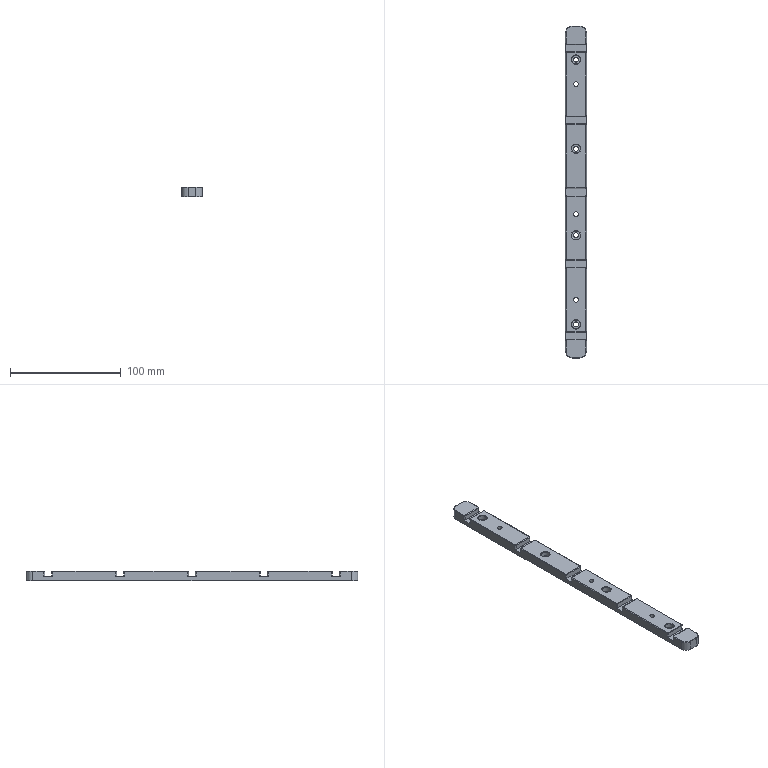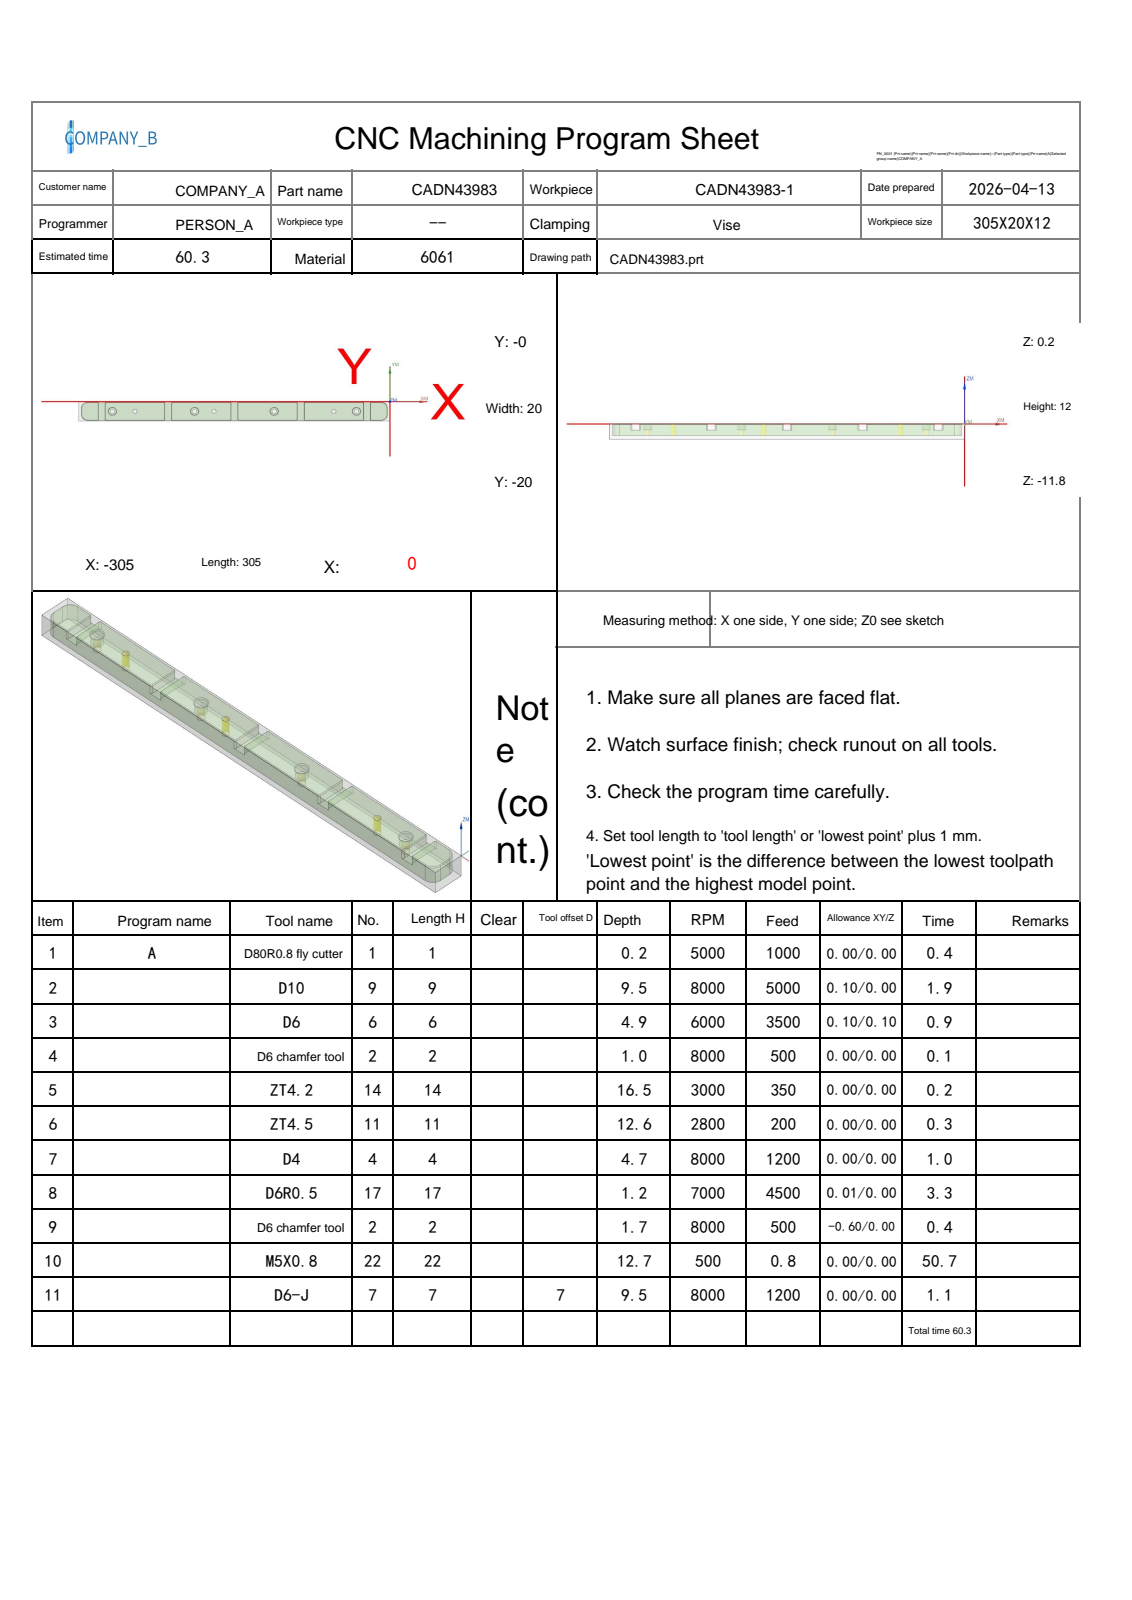NC program | NX | posted by the shop | part box 19 x 300 x 9 mm
Lines 1454 to 2850 of 20188:
N8 T17 M06
(D6R0.5  D=6. R=0.5 H=17 ce=0.01 di=0.00)
G00 G90 G54 X-.332 Y-12.302 M03 S7000
G43 H17 Z20.
M08
Z1.5
G01 Y-13.5 Z1.437 F4500.
Y-13.786 Z1.422
X-.395 Y-14.549 Z1.382
X-.529 Y-15.304 Z1.342
X-.733 Y-16.043 Z1.302
X-1.005 Y-16.759 Z1.262
X-1.344 Y-17.447 Z1.221
X-1.745 Y-18.1 Z1.181
X-2.205 Y-18.712 Z1.141
X-2.721 Y-19.279 Z1.101
X-3.288 Y-19.795 Z1.061
X-3.9 Y-20.255 Z1.021
X-4.553 Y-20.656 Z.98
X-5.241 Y-20.995 Z.94
X-5.957 Y-21.267 Z.9
X-6.696 Y-21.471 Z.86
X-7.45 Y-21.605 Z.82
X-8.214 Y-21.668 Z.78
X-18.528 Z.239
X-18.986 Y-21.608 Z.215
X-19.431 Y-21.482 Z.191
X-19.853 Y-21.294 Z.166
X-20.243 Y-21.046 Z.142
X-20.593 Y-20.743 Z.118
X-20.896 Y-20.393 Z.094
X-21.144 Y-20.003 Z.07
X-21.332 Y-19.581 Z.045
X-21.458 Y-19.136 Z.021
X-21.518 Y-18.678 Z-.003
Y-18.5 Z-.012
Y-1.5
G02 X-18.35 Y1.668 I3.168 J0.0
G01 X-8.5
G02 X-.332 Y-6.5 I0.0 J-8.168
G01 Y-13.5
G02 X-8.5 Y-21.668 I-8.168 J0.0
G01 X-18.35
G02 X-21.518 Y-18.5 I0.0 J3.168
G01 X-21.521 Y-15.667 Z-.013
X-21.527 Y-12.833 Z-.014
X-21.53 Y-10. Z-.015
X-21.536 Y-7.167 Z-.016
X-21.54 Y-4.333
X-21.544 Y-1.5 Z-.017
X-21.543 Y-1.41
X-21.539 Y-1.321
X-21.533 Y-1.231
X-21.524 Y-1.142
X-21.514 Y-1.053
X-21.499 Y-.965
X-21.484 Y-.877
X-21.465 Y-.789
X-21.444 Y-.702
X-21.42 Y-.616
X-21.395 Y-.53
X-21.366 Y-.445
X-21.336 Y-.36 Z-.018
X-21.302 Y-.277
X-21.268 Y-.194
X-21.229 Y-.113
X-21.19 Y-.033
X-21.147 Y.046
X-21.103 Y.124
X-21.056 Y.201
X-21.008 Y.276
X-20.957 Y.35
X-20.905 Y.423
X-20.849 Y.493
X-20.793 Y.563
X-20.734 Y.63
X-20.674 Y.697
X-20.611 Y.761
X-20.547 Y.824
X-20.481 Y.884
X-20.413 Y.944
X-20.344 Y1.
X-20.273 Y1.056
X-20.201 Y1.108
X-20.127 Y1.16
X-20.052 Y1.208
X-19.975 Y1.255
X-19.897 Y1.299
X-19.818 Y1.342
X-19.738 Y1.382
X-19.657 Y1.421
X-19.574 Y1.456
X-19.491 Y1.489
X-19.407 Y1.52
X-19.322 Y1.549
X-19.236 Y1.575
X-19.149 Y1.599
X-19.062 Y1.62
X-18.974 Y1.639
X-18.886 Y1.655
X-18.797 Y1.669
X-18.708 Y1.68
X-18.619 Y1.69
X-18.529 Y1.696 Z-.019
X-18.44 Y1.7
X-18.35 Y1.701
X-15.888 Y1.705
X-13.425 Y1.708 Z-.02
X-10.963 Y1.712 Z-.021
X-8.5 Y1.715
X-8.22 Y1.71
X-7.939 Y1.697
X-7.66 Y1.673 Z-.022
X-7.381 Y1.64
X-7.104 Y1.597
X-6.828 Y1.545
X-6.554 Y1.484
X-6.283 Y1.413
X-6.014 Y1.333
X-5.748 Y1.244
X-5.485 Y1.146
X-5.225 Y1.039
X-4.97 Y.923
X-4.718 Y.799
X-4.471 Y.665
X-4.229 Y.524 Z-.023
X-3.991 Y.374
X-3.759 Y.217
X-3.532 Y.051
X-3.311 Y-.122
X-3.096 Y-.303
X-2.887 Y-.49
X-2.685 Y-.685
X-2.49 Y-.887
X-2.302 Y-1.095
X-2.12 Y-1.31
X-1.947 Y-1.53
X-1.781 Y-1.757
X-1.622 Y-1.989 Z-.024
X-1.472 Y-2.226
X-1.33 Y-2.468
X-1.196 Y-2.715
X-1.071 Y-2.967
X-.954 Y-3.222
X-.846 Y-3.482
X-.748 Y-3.745
X-.701 Y-3.877
X-.657 Y-4.011
X-.616 Y-4.145
X-.577 Y-4.28
X-.54 Y-4.416
X-.505 Y-4.552
X-.473 Y-4.688
X-.443 Y-4.826
X-.415 Y-4.964
X-.39 Y-5.102
X-.367 Y-5.24 Z-.025
X-.347 Y-5.379
X-.329 Y-5.519
X-.313 Y-5.658
X-.3 Y-5.798
X-.289 Y-5.938
X-.28 Y-6.079
X-.274 Y-6.219
X-.27 Y-6.359
X-.269 Y-6.5
X-.267 Y-8.25
X-.265 Y-10. Z-.026
X-.263 Y-11.75
X-.261 Y-13.5 Z-.027
Y-13.641
X-.265 Y-13.781
X-.271 Y-13.922
X-.279 Y-14.062
X-.29 Y-14.203
X-.303 Y-14.343
X-.318 Y-14.482
X-.336 Y-14.622
X-.356 Y-14.761
X-.379 Y-14.9
X-.404 Y-15.039
X-.431 Y-15.177
X-.46 Y-15.314
X-.493 Y-15.451
X-.527 Y-15.588
X-.564 Y-15.724
X-.602 Y-15.859
X-.644 Y-15.993
X-.687 Y-16.127 Z-.028
X-.733 Y-16.26
X-.781 Y-16.393
X-.832 Y-16.524
X-.884 Y-16.655
X-.939 Y-16.784
X-.996 Y-16.913
X-1.055 Y-17.041
X-1.117 Y-17.167
X-1.18 Y-17.293
X-1.246 Y-17.417
X-1.314 Y-17.541
X-1.383 Y-17.663
X-1.456 Y-17.784
X-1.529 Y-17.904
X-1.606 Y-18.022
X-1.684 Y-18.139
X-1.764 Y-18.255
X-1.846 Y-18.369
X-1.93 Y-18.482
X-2.016 Y-18.594
X-2.104 Y-18.704
X-2.193 Y-18.813
X-2.285 Y-18.92
X-2.378 Y-19.025
X-2.473 Y-19.129
X-2.57 Y-19.231 Z-.029
X-2.668 Y-19.331
X-2.769 Y-19.43
X-2.871 Y-19.527
X-2.974 Y-19.623
X-3.08 Y-19.716
X-3.186 Y-19.808
X-3.295 Y-19.898
X-3.516 Y-20.072
X-3.743 Y-20.239
X-3.976 Y-20.398
X-4.214 Y-20.548
X-4.457 Y-20.691
X-4.705 Y-20.825
X-4.957 Y-20.951
X-5.213 Y-21.067
X-5.473 Y-21.176 Z-.03
X-5.737 Y-21.275
X-6.004 Y-21.365
X-6.274 Y-21.446
X-6.546 Y-21.517
X-6.821 Y-21.58
X-7.098 Y-21.633
X-7.376 Y-21.676
X-7.656 Y-21.71
X-7.937 Y-21.735
X-8.218 Y-21.749
X-8.5 Y-21.754
X-10.963 Y-21.757 Z-.031
X-13.425 Y-21.76 Z-.032
X-15.888 Y-21.762
X-18.35 Y-21.765 Z-.033
X-18.442 Y-21.764
X-18.533 Y-21.76
X-18.624 Y-21.754
X-18.716 Y-21.744
X-18.806 Y-21.733
X-18.897 Y-21.719
X-18.987 Y-21.703
X-19.077 Y-21.683
X-19.166 Y-21.662
X-19.254 Y-21.638
X-19.342 Y-21.612
X-19.429 Y-21.582
X-19.515 Y-21.551
X-19.6 Y-21.517
X-19.684 Y-21.481
X-19.767 Y-21.443
X-19.849 Y-21.402 Z-.034
X-19.93 Y-21.359
X-20.01 Y-21.314
X-20.088 Y-21.266
X-20.165 Y-21.216
X-20.24 Y-21.164
X-20.315 Y-21.11
X-20.387 Y-21.054
X-20.458 Y-20.996
X-20.527 Y-20.936
X-20.595 Y-20.874
X-20.66 Y-20.81
X-20.725 Y-20.745
X-20.786 Y-20.677
X-20.847 Y-20.608
X-20.905 Y-20.537
X-20.961 Y-20.465
X-21.015 Y-20.391
X-21.067 Y-20.316
X-21.117 Y-20.239
X-21.165 Y-20.161
X-21.21 Y-20.081
X-21.254 Y-20.
X-21.295 Y-19.918
X-21.334 Y-19.835
X-21.37 Y-19.751
X-21.404 Y-19.666
X-21.435 Y-19.58
X-21.465 Y-19.493
X-21.491 Y-19.405
X-21.516 Y-19.317
X-21.537 Y-19.227
X-21.557 Y-19.138
X-21.573 Y-19.048
X-21.588 Y-18.957
X-21.599 Y-18.866
X-21.608 Y-18.775
X-21.614 Y-18.683
X-21.619 Y-18.592
X-21.62 Y-18.5 Z-.035
X-21.624 Y-15.667 Z-.036
X-21.628 Y-12.833 Z-.037
X-21.631 Y-10. Z-.038
X-21.636 Y-7.167 Z-.039
X-21.64 Y-4.333 Z-.04
X-21.644 Y-1.5 Z-.041
X-21.639 Y-1.328
X-21.626 Y-1.156
X-21.604 Y-.985
X-21.572 Y-.815
X-21.533 Y-.647 Z-.042
X-21.484 Y-.482
X-21.426 Y-.319
X-21.36 Y-.16
X-21.287 Y-.004
X-21.204 Y.148
X-21.114 Y.295
X-21.017 Y.438
X-20.912 Y.575
X-20.8 Y.706
X-20.681 Y.831
X-20.556 Y.95
X-20.425 Y1.063
X-20.288 Y1.168
X-20.146 Y1.266 Z-.043
X-19.999 Y1.356
X-19.848 Y1.439
X-19.692 Y1.513
X-19.532 Y1.58
X-19.369 Y1.638
X-19.204 Y1.687
X-19.036 Y1.727
X-18.866 Y1.759
X-18.695 Y1.782
X-18.523 Y1.796
X-18.35 Y1.801
X-15.888 Y1.803 Z-.044
X-13.425 Y1.807 Z-.045
X-10.963 Y1.81 Z-.046
X-8.5 Y1.813 Z-.047
X-8.216 Y1.809
X-7.933 Y1.794
X-7.65 Y1.771
X-7.368 Y1.737 Z-.048
X-7.087 Y1.694
X-6.808 Y1.641
X-6.531 Y1.579
X-6.256 Y1.508
X-5.984 Y1.427
X-5.715 Y1.337
X-5.449 Y1.237
X-5.186 Y1.129
X-4.928 Y1.012 Z-.049
X-4.673 Y.886
X-4.423 Y.751
X-4.178 Y.608
X-3.937 Y.456
X-3.702 Y.297
X-3.473 Y.129
X-3.249 Y-.046
X-3.032 Y-.229 Z-.05
X-2.82 Y-.419
X-2.616 Y-.616
X-2.418 Y-.82
X-2.228 Y-1.031
X-2.044 Y-1.248
X-1.869 Y-1.471
X-1.7 Y-1.7
X-1.54 Y-1.935
X-1.388 Y-2.175 Z-.051
X-1.244 Y-2.42
X-1.109 Y-2.67
X-.982 Y-2.925
X-.864 Y-3.183
X-.755 Y-3.446
X-.655 Y-3.712
X-.564 Y-3.981
X-.483 Y-4.254
X-.41 Y-4.529 Z-.052
X-.347 Y-4.806
X-.294 Y-5.085
X-.25 Y-5.366
X-.232 Y-5.507
X-.216 Y-5.648
X-.202 Y-5.79
X-.191 Y-5.932
X-.182 Y-6.074
X-.176 Y-6.216
X-.172 Y-6.358
X-.171 Y-6.5
X-.169 Y-8.25 Z-.053
X-.167 Y-10. Z-.054
X-.165 Y-11.75
X-.163 Y-13.5 Z-.055
X-.164 Y-13.642
X-.168 Y-13.785
X-.173 Y-13.927
X-.182 Y-14.069
X-.192 Y-14.211
X-.206 Y-14.353
X-.221 Y-14.494
X-.24 Y-14.635 Z-.056
X-.26 Y-14.776
X-.283 Y-14.917
X-.308 Y-15.057
X-.336 Y-15.197
X-.365 Y-15.336
X-.398 Y-15.474
X-.433 Y-15.613
X-.47 Y-15.75
X-.509 Y-15.887
X-.551 Y-16.023
X-.595 Y-16.158
X-.642 Y-16.293
X-.69 Y-16.427
X-.741 Y-16.56
X-.794 Y-16.692
X-.85 Y-16.823
X-.907 Y-16.953
X-.967 Y-17.082 Z-.057
X-1.029 Y-17.211
X-1.094 Y-17.338
X-1.16 Y-17.464
X-1.229 Y-17.588
X-1.299 Y-17.712
X-1.373 Y-17.834
X-1.447 Y-17.956
X-1.524 Y-18.075
X-1.603 Y-18.194
X-1.684 Y-18.311
X-1.767 Y-18.427
X-1.852 Y-18.541
X-1.939 Y-18.654
X-2.028 Y-18.765
X-2.119 Y-18.875
X-2.211 Y-18.984
X-2.306 Y-19.09
X-2.402 Y-19.195 Z-.058
X-2.5 Y-19.299
X-2.6 Y-19.4
X-2.701 Y-19.5
X-2.804 Y-19.598
X-2.909 Y-19.695
X-3.016 Y-19.79
X-3.124 Y-19.883
X-3.233 Y-19.973
X-3.345 Y-20.063
X-3.457 Y-20.15
X-3.571 Y-20.235
X-3.687 Y-20.318
X-3.804 Y-20.4
X-3.922 Y-20.479
X-4.042 Y-20.556
X-4.163 Y-20.631
X-4.286 Y-20.705 Z-.059
X-4.409 Y-20.776
X-4.534 Y-20.845
X-4.66 Y-20.911
X-4.915 Y-21.038
X-5.174 Y-21.157
X-5.437 Y-21.266
X-5.704 Y-21.366
X-5.974 Y-21.458
X-6.247 Y-21.539
X-6.523 Y-21.612
X-6.801 Y-21.675 Z-.06
X-7.081 Y-21.729
X-7.363 Y-21.773
X-7.646 Y-21.807
X-7.93 Y-21.832
X-8.215 Y-21.846
X-8.5 Y-21.852
X-10.963 Y-21.854 Z-.061
X-13.425 Y-21.857 Z-.062
X-15.888 Y-21.859 Z-.063
X-18.35 Y-21.862 Z-.064
X-18.526 Y-21.858
X-18.701 Y-21.844
X-18.876 Y-21.821
X-19.049 Y-21.789
X-19.22 Y-21.748
X-19.389 Y-21.699 Z-.065
X-19.555 Y-21.64
X-19.718 Y-21.573
X-19.877 Y-21.497
X-20.032 Y-21.413
X-20.182 Y-21.321
X-20.327 Y-21.222
X-20.467 Y-21.115
X-20.601 Y-21.
X-20.729 Y-20.879
X-20.851 Y-20.752
X-20.965 Y-20.618
X-21.073 Y-20.478
X-21.173 Y-20.333
X-21.265 Y-20.183 Z-.066
X-21.349 Y-20.028
X-21.425 Y-19.869
X-21.493 Y-19.706
X-21.552 Y-19.54
X-21.602 Y-19.371
X-21.643 Y-19.2
X-21.676 Y-19.027
X-21.699 Y-18.852
X-21.713 Y-18.676
X-21.718 Y-18.5
X-21.721 Y-15.667 Z-.068
X-21.725 Y-12.833 Z-.069
X-21.729 Y-10. Z-.071
X-21.732 Y-7.167 Z-.072
X-21.736 Y-4.333 Z-.073
X-21.739 Y-1.5 Z-.075
X-21.735 Y-1.323
X-21.721 Y-1.146
X-21.698 Y-.97
X-21.666 Y-.795
X-21.625 Y-.622
X-21.575 Y-.452
X-21.516 Y-.285
X-21.448 Y-.121 Z-.076
X-21.372 Y.04
X-21.287 Y.196
X-21.195 Y.347
X-21.094 Y.494
X-20.986 Y.635
X-20.871 Y.77
X-20.749 Y.899
X-20.62 Y1.021
X-20.485 Y1.137
X-20.344 Y1.245
X-20.198 Y1.346 Z-.077
X-20.047 Y1.439
X-19.891 Y1.524
X-19.73 Y1.6
X-19.566 Y1.669
X-19.399 Y1.728
X-19.229 Y1.779
X-19.056 Y1.821
X-18.881 Y1.853
X-18.705 Y1.877
X-18.528 Y1.891
X-18.35 Y1.896 Z-.078
X-15.888 Y1.898 Z-.079
X-13.425 Y1.902 Z-.08
X-10.963 Y1.904 Z-.081
X-8.5 Y1.908 Z-.083
X-8.213 Y1.903
X-7.926 Y1.889
X-7.64 Y1.865
X-7.355 Y1.831
X-7.071 Y1.787
X-6.789 Y1.734
X-6.509 Y1.671 Z-.084
X-6.231 Y1.598
X-5.956 Y1.517
X-5.683 Y1.425
X-5.414 Y1.325
X-5.149 Y1.215
X-4.887 Y1.097
X-4.63 Y.969 Z-.085
X-4.377 Y.833
X-4.129 Y.688
X-3.886 Y.535
X-3.648 Y.374
X-3.416 Y.204
X-3.19 Y.027
X-2.97 Y-.158 Z-.086
X-2.756 Y-.35
X-2.55 Y-.55
X-2.349 Y-.756
X-2.157 Y-.969
X-1.971 Y-1.189
X-1.794 Y-1.414
X-1.624 Y-1.646 Z-.087
X-1.462 Y-1.884
X-1.308 Y-2.126
X-1.162 Y-2.374
X-1.026 Y-2.627
X-.897 Y-2.884
X-.778 Y-3.146
X-.668 Y-3.411 Z-.088
X-.567 Y-3.68
X-.475 Y-3.953
X-.392 Y-4.228
X-.319 Y-4.506
X-.255 Y-4.787
X-.201 Y-5.069 Z-.089
X-.157 Y-5.353
X-.122 Y-5.639
X-.098 Y-5.925
X-.089 Y-6.069
X-.083 Y-6.212
X-.079 Y-6.356
X-.077 Y-6.5
X-.075 Y-8.25 Z-.09
X-.074 Y-10. Z-.091
X-.071 Y-11.75 Z-.092
X-.07 Y-13.5 Z-.093
X-.071 Y-13.644
X-.074 Y-13.788
X-.08 Y-13.932
X-.089 Y-14.075
X-.099 Y-14.219
X-.113 Y-14.362
X-.129 Y-14.505
X-.147 Y-14.648
X-.167 Y-14.791
X-.191 Y-14.933 Z-.094
X-.216 Y-15.074
X-.244 Y-15.215
X-.274 Y-15.356
X-.307 Y-15.496
X-.342 Y-15.636
X-.38 Y-15.775
X-.42 Y-15.914
X-.462 Y-16.051
X-.506 Y-16.188
X-.554 Y-16.324
X-.603 Y-16.46
X-.654 Y-16.594
X-.708 Y-16.728
X-.764 Y-16.86 Z-.095
X-.822 Y-16.992
X-.883 Y-17.122
X-.946 Y-17.252
X-1.011 Y-17.38
X-1.078 Y-17.508
X-1.147 Y-17.634
X-1.219 Y-17.759
X-1.293 Y-17.883
X-1.368 Y-18.005
X-1.446 Y-18.127
X-1.526 Y-18.246
X-1.608 Y-18.365
X-1.692 Y-18.482
X-1.778 Y-18.598 Z-.096
X-1.866 Y-18.712
X-1.956 Y-18.824
X-2.047 Y-18.935
X-2.141 Y-19.045
X-2.236 Y-19.153
X-2.334 Y-19.259
X-2.433 Y-19.363
X-2.534 Y-19.466
X-2.636 Y-19.567
X-2.741 Y-19.667
X-2.847 Y-19.764
X-2.954 Y-19.86
X-3.064 Y-19.954 Z-.097
X-3.175 Y-20.046
X-3.287 Y-20.136
X-3.401 Y-20.224
X-3.516 Y-20.31
X-3.633 Y-20.394
X-3.752 Y-20.477
X-3.871 Y-20.557
X-3.992 Y-20.635
X-4.115 Y-20.711
X-4.239 Y-20.785
X-4.363 Y-20.857
X-4.49 Y-20.927
X-4.617 Y-20.994
X-4.745 Y-21.059 Z-.098
X-4.875 Y-21.123
X-5.005 Y-21.184
X-5.137 Y-21.242
X-5.27 Y-21.299
X-5.403 Y-21.353
X-5.538 Y-21.405
X-5.673 Y-21.454
X-5.809 Y-21.501
X-5.946 Y-21.546
X-6.084 Y-21.589
X-6.222 Y-21.629
X-6.361 Y-21.667
X-6.501 Y-21.702
X-6.641 Y-21.736 Z-.099
X-6.782 Y-21.766
X-6.924 Y-21.795
X-7.065 Y-21.82
X-7.208 Y-21.844
X-7.35 Y-21.865
X-7.637 Y-21.899
X-7.924 Y-21.924
X-8.212 Y-21.939
X-8.5 Y-21.945 Z-.1
X-10.963 Y-21.947 Z-.101
X-13.425 Y-21.95 Z-.102
X-15.888 Y-21.952 Z-.103
X-18.35 Y-21.955 Z-.104
X-18.531 Y-21.95 Z-.105
X-18.711 Y-21.936
X-18.891 Y-21.913
X-19.068 Y-21.88
X-19.244 Y-21.838
X-19.418 Y-21.787
X-19.589 Y-21.727
X-19.756 Y-21.657
X-19.919 Y-21.58
X-20.078 Y-21.494
X-20.233 Y-21.399 Z-.106
X-20.382 Y-21.297
X-20.526 Y-21.187
X-20.663 Y-21.069
X-20.795 Y-20.945
X-20.92 Y-20.814
X-21.037 Y-20.676
X-21.148 Y-20.533
X-21.25 Y-20.383
X-21.345 Y-20.229
X-21.432 Y-20.07
X-21.51 Y-19.907 Z-.107
X-21.579 Y-19.74
X-21.64 Y-19.569
X-21.691 Y-19.395
X-21.734 Y-19.219
X-21.767 Y-19.041
X-21.791 Y-18.862
X-21.805 Y-18.681
X-21.811 Y-18.5
X-21.814 Y-15.667 Z-.109
X-21.817 Y-12.833 Z-.111
X-21.82 Y-10. Z-.112
X-21.824 Y-7.167 Z-.114
X-21.827 Y-4.333 Z-.116
X-21.83 Y-1.5 Z-.118
X-21.826 Y-1.318
X-21.812 Y-1.136
X-21.788 Y-.955
X-21.755 Y-.776
X-21.713 Y-.599
X-21.661 Y-.424
X-21.601 Y-.252
X-21.531 Y-.084 Z-.119
X-21.453 Y.081
X-21.366 Y.241
X-21.271 Y.397
X-21.168 Y.547
X-21.057 Y.692
X-20.938 Y.831
X-20.813 Y.963
X-20.681 Y1.089
X-20.542 Y1.207 Z-.12
X-20.398 Y1.319
X-20.248 Y1.422
X-20.092 Y1.518
X-19.932 Y1.605
X-19.767 Y1.683
X-19.599 Y1.754
X-19.427 Y1.815
X-19.252 Y1.867
X-19.075 Y1.909 Z-.121
X-18.895 Y1.943
X-18.714 Y1.967
X-18.532 Y1.982
X-18.35 Y1.986
X-15.888 Y1.989 Z-.123
X-13.425 Y1.992 Z-.124
X-10.963 Y1.995 Z-.126
X-8.5 Y1.998 Z-.127
X-8.21 Y1.993
X-7.92 Y1.978
X-7.631 Y1.954 Z-.128
X-7.343 Y1.92
X-7.056 Y1.876
X-6.771 Y1.822
X-6.488 Y1.758
X-6.207 Y1.685
X-5.928 Y1.602 Z-.129
X-5.653 Y1.51
X-5.381 Y1.408
X-5.113 Y1.298
X-4.849 Y1.178
X-4.588 Y1.049 Z-.13
X-4.333 Y.911
X-4.082 Y.765
X-3.837 Y.61
X-3.596 Y.447
X-3.362 Y.276
X-3.133 Y.097 Z-.131
X-2.911 Y-.09
X-2.695 Y-.284
X-2.486 Y-.486
X-2.284 Y-.695
X-2.089 Y-.91
X-1.902 Y-1.132 Z-.132
X-1.722 Y-1.36
X-1.55 Y-1.594
X-1.387 Y-1.834
X-1.231 Y-2.08
X-1.085 Y-2.33 Z-.133
X-.946 Y-2.586
X-.817 Y-2.846
X-.696 Y-3.11
X-.585 Y-3.379
X-.482 Y-3.651
X-.39 Y-3.926 Z-.134
X-.306 Y-4.204
X-.232 Y-4.485
X-.168 Y-4.769
X-.113 Y-5.054
X-.069 Y-5.341 Z-.135
X-.05 Y-5.485
X-.034 Y-5.63
X-.02 Y-5.774
X-.009 Y-5.919
X0.0 Y-6.064
X.007 Y-6.209
X.011 Y-6.355
X.012 Y-6.5
X.014 Y-8.25 Z-.136
X.015 Y-10. Z-.137
X.018 Y-11.75 Z-.138
X.019 Y-13.5 Z-.14
X.018 Y-13.645
X.015 Y-13.791
X.009 Y-13.936
X0.0 Y-14.081
X-.011 Y-14.227
X-.025 Y-14.371
X-.04 Y-14.516
X-.059 Y-14.66
X-.08 Y-14.804
X-.103 Y-14.948
X-.129 Y-15.091
X-.157 Y-15.234 Z-.141
X-.188 Y-15.376
X-.221 Y-15.518
X-.256 Y-15.659
X-.295 Y-15.799
X-.335 Y-15.939
X-.377 Y-16.078
X-.422 Y-16.216
X-.47 Y-16.354
X-.52 Y-16.491
X-.572 Y-16.627
X-.626 Y-16.761 Z-.142
X-.683 Y-16.895
X-.742 Y-17.029
X-.803 Y-17.161
X-.866 Y-17.291
X-.932 Y-17.421
X-1. Y-17.55
X-1.07 Y-17.678
X-1.142 Y-17.804
X-1.217 Y-17.929
X-1.293 Y-18.053
X-1.372 Y-18.175 Z-.143
X-1.453 Y-18.296
X-1.536 Y-18.416
X-1.62 Y-18.534
X-1.707 Y-18.651
X-1.796 Y-18.766
X-1.887 Y-18.88
X-1.98 Y-18.992
X-2.074 Y-19.103
X-2.171 Y-19.212
X-2.269 Y-19.319
X-2.369 Y-19.425 Z-.144
X-2.471 Y-19.529
X-2.575 Y-19.631
X-2.68 Y-19.731
X-2.787 Y-19.83
X-2.896 Y-19.927
X-3.007 Y-20.022
X-3.119 Y-20.114
X-3.232 Y-20.206
X-3.348 Y-20.295
X-3.464 Y-20.382
X-3.582 Y-20.467 Z-.145
X-3.702 Y-20.55
X-3.823 Y-20.631
X-3.945 Y-20.71
X-4.069 Y-20.786
X-4.194 Y-20.861
X-4.32 Y-20.934
X-4.448 Y-21.004
X-4.576 Y-21.072
X-4.706 Y-21.139
X-4.837 Y-21.202
X-4.969 Y-21.264
X-5.102 Y-21.323 Z-.146
X-5.236 Y-21.38
X-5.371 Y-21.435
X-5.507 Y-21.487
X-5.644 Y-21.537
X-5.781 Y-21.585
X-5.919 Y-21.631
X-6.059 Y-21.674
X-6.199 Y-21.714
X-6.339 Y-21.752
X-6.48 Y-21.788
X-6.622 Y-21.822 Z-.147
X-6.764 Y-21.853
X-6.907 Y-21.881
X-7.05 Y-21.907
X-7.194 Y-21.931
X-7.338 Y-21.952
X-7.483 Y-21.971
X-7.627 Y-21.987
X-7.772 Y-22.001
X-7.918 Y-22.012
X-8.063 Y-22.021
X-8.209 Y-22.028 Z-.148
X-8.354 Y-22.032
X-8.5 Y-22.033
X-10.963 Y-22.035 Z-.149
X-13.425 Y-22.038 Z-.151
X-15.888 Y-22.04 Z-.152
X-18.35 Y-22.043 Z-.154
X-18.535 Y-22.038
X-18.72 Y-22.024
X-18.904 Y-21.999
X-19.087 Y-21.966
X-19.267 Y-21.923
X-19.445 Y-21.87
X-19.62 Y-21.808 Z-.155
X-19.792 Y-21.738
X-19.959 Y-21.658
X-20.122 Y-21.57
X-20.28 Y-21.473
X-20.434 Y-21.368
X-20.581 Y-21.255
X-20.722 Y-21.135
X-20.857 Y-21.007
X-20.985 Y-20.872 Z-.156
X-21.105 Y-20.731
X-21.219 Y-20.584
X-21.324 Y-20.431
X-21.421 Y-20.273
X-21.51 Y-20.11
X-21.59 Y-19.942
X-21.661 Y-19.771
X-21.723 Y-19.596
X-21.776 Y-19.418 Z-.157
X-21.82 Y-19.238
X-21.854 Y-19.055
X-21.878 Y-18.871
X-21.893 Y-18.686
X-21.898 Y-18.5
X-21.901 Y-15.667 Z-.159
X-21.904 Y-12.833 Z-.161
X-21.907 Y-10. Z-.163
X-21.91 Y-7.167 Z-.165
X-21.913 Y-4.333 Z-.167
X-21.916 Y-1.5 Z-.169
X-21.912 Y-1.313
X-21.897 Y-1.127 Z-.17
X-21.873 Y-.942
X-21.839 Y-.758
X-21.796 Y-.577
X-21.743 Y-.398
X-21.681 Y-.221
X-21.609 Y-.049
X-21.57 Y.036
X-21.529 Y.12
X-21.486 Y.203 Z-.171
X-21.44 Y.284
X-21.393 Y.365
X-21.343 Y.444
X-21.291 Y.521
X-21.237 Y.598
X-21.181 Y.673
X-21.124 Y.746
X-21.064 Y.818
X-21.002 Y.888
X-20.939 Y.957
X-20.874 Y1.024
X-20.807 Y1.089
X-20.738 Y1.153
X-20.668 Y1.214
X-20.596 Y1.274 Z-.172
X-20.523 Y1.332
X-20.448 Y1.388
X-20.372 Y1.442
X-20.294 Y1.494
X-20.215 Y1.544
X-20.135 Y1.592
X-20.054 Y1.638
X-19.971 Y1.681
X-19.887 Y1.723
X-19.802 Y1.762
X-19.716 Y1.799
X-19.63 Y1.834
X-19.542 Y1.866
X-19.453 Y1.896
X-19.364 Y1.924
X-19.274 Y1.95 Z-.173
X-19.184 Y1.973
X-19.093 Y1.993
X-19.001 Y2.012
X-18.909 Y2.028
X-18.816 Y2.041
X-18.723 Y2.052
X-18.63 Y2.061
X-18.537 Y2.067
X-18.444 Y2.071
X-18.35 Y2.072
X-15.888 Y2.074 Z-.175
X-13.425 Y2.077 Z-.177
X-10.963 Y2.08 Z-.178
X-8.5 Y2.082 Z-.18
X-8.353
X-8.207 Y2.078
X-8.061 Y2.072 Z-.181
X-7.914 Y2.063
X-7.768 Y2.052
X-7.622 Y2.038
X-7.477 Y2.022
X-7.331 Y2.004
X-7.186 Y1.983
X-7.041 Y1.959
X-6.897 Y1.933
X-6.753 Y1.905
X-6.61 Y1.874 Z-.182
X-6.467 Y1.841
X-6.325 Y1.805
X-6.184 Y1.767
X-6.043 Y1.726
X-5.903 Y1.683
X-5.763 Y1.638
X-5.625 Y1.59
X-5.487 Y1.54
X-5.35 Y1.487 Z-.183
X-5.214 Y1.432
X-5.079 Y1.375
X-4.945 Y1.316
X-4.812 Y1.254
X-4.68 Y1.19
X-4.55 Y1.124
X-4.42 Y1.056
X-4.291 Y.985
X-4.164 Y.912
X-4.038 Y.837 Z-.184
X-3.913 Y.76
X-3.79 Y.681
X-3.668 Y.6
X-3.547 Y.516
X-3.428 Y.431
X-3.311 Y.343
X-3.194 Y.254
X-3.08 Y.162
X-2.967 Y.069 Z-.185
X-2.855 Y-.026
X-2.746 Y-.124
X-2.637 Y-.223
X-2.531 Y-.324
X-2.426 Y-.426
X-2.323 Y-.531
X-2.222 Y-.637
X-2.123 Y-.745
X-2.026 Y-.855
X-1.93 Y-.966 Z-.186
X-1.836 Y-1.079
X-1.745 Y-1.193
X-1.655 Y-1.309
X-1.567 Y-1.427
X-1.482 Y-1.546
X-1.398 Y-1.666
X-1.316 Y-1.788
X-1.237 Y-1.911
X-1.159 Y-2.036
X-1.084 Y-2.162 Z-.187
X-1.011 Y-2.289
X-.94 Y-2.417
X-.871 Y-2.547
X-.805 Y-2.678
X-.741 Y-2.81
X-.678 Y-2.943
X-.619 Y-3.077
X-.561 Y-3.212
X-.506 Y-3.348 Z-.188
X-.453 Y-3.485
X-.403 Y-3.622
X-.355 Y-3.761
X-.309 Y-3.9
X-.266 Y-4.041
X-.225 Y-4.181
X-.186 Y-4.323
X-.15 Y-4.465
X-.117 Y-4.608
X-.086 Y-4.751 Z-.189
X-.057 Y-4.895
X-.03 Y-5.04
X-.006 Y-5.184
X.015 Y-5.33
X.034 Y-5.475
X.05 Y-5.621
X.064 Y-5.767
X.075 Y-5.913
X.084 Y-6.06 Z-.19
X.091 Y-6.207
X.095 Y-6.353
X.096 Y-6.5
X.098 Y-8.25 Z-.191
X.099 Y-10. Z-.192
X.101 Y-11.75 Z-.194
X.103 Y-13.5 Z-.195
X.102 Y-13.647
X.098 Y-13.794
X.092 Y-13.94
X.083 Y-14.087
X.072 Y-14.233
X.058 Y-14.38
X.043 Y-14.526 Z-.196
X.024 Y-14.671
X.003 Y-14.817
X-.021 Y-14.962
X-.047 Y-15.106
X-.076 Y-15.25
X-.106 Y-15.394
X-.14 Y-15.537
X-.176 Y-15.68
X-.214 Y-15.821
X-.255 Y-15.963 Z-.197
X-.298 Y-16.103
X-.343 Y-16.243
X-.391 Y-16.382
X-.441 Y-16.52
X-.494 Y-16.657
X-.549 Y-16.793
X-.606 Y-16.928
X-.666 Y-17.063
X-.728 Y-17.196 Z-.198
X-.792 Y-17.328
X-.858 Y-17.459
X-.927 Y-17.59
X-.998 Y-17.718
X-1.07 Y-17.846
X-1.146 Y-17.972
X-1.223 Y-18.097
X-1.303 Y-18.221
X-1.384 Y-18.343
X-1.468 Y-18.464 Z-.199
X-1.553 Y-18.583
X-1.641 Y-18.701
X-1.731 Y-18.818
X-1.822 Y-18.932
X-1.916 Y-19.046
X-2.012 Y-19.157
X-2.109 Y-19.268
X-2.208 Y-19.376
X-2.309 Y-19.483 Z-.2
X-2.412 Y-19.587
X-2.517 Y-19.691
X-2.624 Y-19.792
X-2.732 Y-19.892
X-2.842 Y-19.989
X-2.953 Y-20.085
X-3.066 Y-20.179
X-3.181 Y-20.271
X-3.297 Y-20.361
X-3.415 Y-20.449 Z-.201
X-3.534 Y-20.534
X-3.655 Y-20.619
X-3.777 Y-20.7
X-3.901 Y-20.78
X-4.026 Y-20.857
X-4.152 Y-20.933
X-4.279 Y-21.006
X-4.408 Y-21.077
X-4.538 Y-21.146
X-4.669 Y-21.213 Z-.202
X-4.801 Y-21.277
X-4.934 Y-21.34
X-5.069 Y-21.399
X-5.204 Y-21.457
X-5.34 Y-21.512
X-5.478 Y-21.565
X-5.616 Y-21.615
X-5.755 Y-21.664
X-5.894 Y-21.709 Z-.203
X-6.035 Y-21.753
X-6.176 Y-21.794
X-6.318 Y-21.833
X-6.461 Y-21.869
X-6.604 Y-21.903
X-6.747 Y-21.934
X-6.892 Y-21.963
X-7.036 Y-21.989
X-7.181 Y-22.013
X-7.327 Y-22.034 Z-.204
X-7.473 Y-22.053
X-7.619 Y-22.07
X-7.765 Y-22.084
X-7.912 Y-22.095
X-8.059 Y-22.104
X-8.206 Y-22.11
X-8.353 Y-22.114
X-8.5 Y-22.116
X-10.963 Y-22.118 Z-.206
X-13.425 Y-22.12 Z-.208
X-15.888 Y-22.122 Z-.21
X-18.35 Y-22.125 Z-.211
X-18.54 Y-22.12 Z-.212
X-18.729 Y-22.105
X-18.917 Y-22.081
X-19.104 Y-22.046
X-19.288 Y-22.002
X-19.47 Y-21.948
X-19.649 Y-21.885
X-19.825 Y-21.813
X-19.996 Y-21.731 Z-.213
X-20.163 Y-21.641
X-20.325 Y-21.541
X-20.482 Y-21.434
X-20.632 Y-21.319
X-20.777 Y-21.196
X-20.915 Y-21.065
X-21.046 Y-20.927 Z-.214
X-21.169 Y-20.783
X-21.285 Y-20.632
X-21.393 Y-20.476
X-21.492 Y-20.314
X-21.583 Y-20.147
X-21.665 Y-19.976
X-21.738 Y-19.8 Z-.215
X-21.801 Y-19.621
X-21.855 Y-19.439
X-21.9 Y-19.255
X-21.935 Y-19.068
X-21.96 Y-18.879
X-21.975 Y-18.69
X-21.98 Y-18.5
X-21.983 Y-15.667 Z-.218
X-21.986 Y-12.833 Z-.22
X-21.988 Y-10. Z-.222
X-21.991 Y-7.167 Z-.225
X-21.994 Y-4.333 Z-.227
X-21.997 Y-1.5 Z-.229
X-21.996 Y-1.405
X-21.992 Y-1.309
X-21.986 Y-1.214
X-21.977 Y-1.119
X-21.966 Y-1.024
X-21.952 Y-.929 Z-.23
X-21.936 Y-.835
X-21.918 Y-.742
X-21.897 Y-.648
X-21.873 Y-.556
X-21.848 Y-.464
X-21.819 Y-.373
X-21.789 Y-.282
X-21.756 Y-.193
X-21.721 Y-.104
X-21.683 Y-.016
X-21.643 Y.071
X-21.601 Y.156
X-21.556 Y.241 Z-.231
X-21.51 Y.324
X-21.461 Y.407
X-21.41 Y.487
X-21.357 Y.567
X-21.302 Y.645
X-21.245 Y.721
X-21.186 Y.796
X-21.125 Y.87
X-21.062 Y.942
X-20.997 Y1.012
X-20.93 Y1.08
X-20.862 Y1.147
X-20.792 Y1.212 Z-.232
X-20.72 Y1.275
X-20.647 Y1.336
X-20.572 Y1.396
X-20.495 Y1.453
X-20.418 Y1.508
X-20.338 Y1.561
X-20.257 Y1.613
X-20.175 Y1.661
X-20.092 Y1.708
X-20.007 Y1.753
X-19.922 Y1.795
X-19.835 Y1.835
X-19.747 Y1.873 Z-.233
X-19.658 Y1.908
X-19.569 Y1.942
X-19.478 Y1.972
X-19.387 Y2.001
X-19.295 Y2.027
X-19.202 Y2.051
X-19.109 Y2.072
X-19.015 Y2.091
X-18.921 Y2.107
X-18.827 Y2.121
X-18.732 Y2.132
X-18.637 Y2.141
X-18.541 Y2.147 Z-.234
X-18.446 Y2.151
X-18.35 Y2.152
X-15.888 Y2.155 Z-.236
X-13.425 Y2.157 Z-.238
X-10.963 Y2.159 Z-.24
X-8.5 Y2.162 Z-.242
X-8.217 Y2.157
X-7.933 Y2.144
X-7.651 Y2.121
X-7.369 Y2.089
X-7.089 Y2.047 Z-.243
X-6.81 Y1.997
X-6.533 Y1.937
X-6.258 Y1.868
X-5.985 Y1.791 Z-.244
X-5.715 Y1.704
X-5.448 Y1.609
X-5.184 Y1.505
X-4.924 Y1.393 Z-.245
X-4.667 Y1.272
X-4.415 Y1.142
X-4.167 Y1.005
X-3.924 Y.859
X-3.685 Y.706 Z-.246
X-3.452 Y.545
X-3.224 Y.376
X-3.002 Y.2
X-2.785 Y.017 Z-.247
X-2.575 Y-.174
X-2.371 Y-.371
X-2.173 Y-.575
X-1.983 Y-.784
X-1.799 Y-1.001 Z-.248
X-1.622 Y-1.223
X-1.453 Y-1.45
X-1.292 Y-1.683
X-1.138 Y-1.922 Z-.249
X-.992 Y-2.165
X-.854 Y-2.413
X-.724 Y-2.665
X-.602 Y-2.922 Z-.25
X-.489 Y-3.182
X-.385 Y-3.446
X-.289 Y-3.713
X-.202 Y-3.983
X-.123 Y-4.256 Z-.251
X-.054 Y-4.531
X.006 Y-4.808
X.057 Y-5.087
X.099 Y-5.368 Z-.252
X.132 Y-5.65
X.155 Y-5.933
X.169 Y-6.216
X.174 Y-6.5
X.176 Y-8.25 Z-.254
X.177 Y-10. Z-.255
X.179 Y-11.75 Z-.257
X.18 Y-13.5 Z-.258
X.176 Y-13.784
X.162 Y-14.068 Z-.259
X.139 Y-14.351
X.107 Y-14.633
X.066 Y-14.914
X.015 Y-15.194
X-.045 Y-15.471 Z-.26
X-.114 Y-15.747
X-.191 Y-16.02
X-.278 Y-16.291
X-.373 Y-16.559 Z-.261
X-.478 Y-16.823
X-.59 Y-17.084
X-.712 Y-17.341
X-.841 Y-17.594 Z-.262
X-.979 Y-17.842
X-1.125 Y-18.086
X-1.279 Y-18.325
X-1.44 Y-18.559
X-1.61 Y-18.787 Z-.263
X-1.786 Y-19.01
X-1.97 Y-19.227
X-2.16 Y-19.438
X-2.358 Y-19.642 Z-.264
X-2.562 Y-19.84
X-2.772 Y-20.031
X-2.989 Y-20.215
X-3.212 Y-20.392
X-3.44 Y-20.562 Z-.265
X-3.673 Y-20.723
X-3.912 Y-20.878
X-4.156 Y-21.024
X-4.404 Y-21.163 Z-.266
X-4.657 Y-21.293
X-4.914 Y-21.414
X-5.175 Y-21.528
X-5.439 Y-21.633 Z-.267
X-5.707 Y-21.728
X-5.977 Y-21.816
X-6.251 Y-21.894
X-6.527 Y-21.963
X-6.805 Y-22.024 Z-.268
X-7.084 Y-22.075
X-7.366 Y-22.117
X-7.648 Y-22.15
X-7.932 Y-22.173 Z-.269
X-8.216 Y-22.187
X-8.5 Y-22.192
X-10.963 Y-22.194 Z-.271